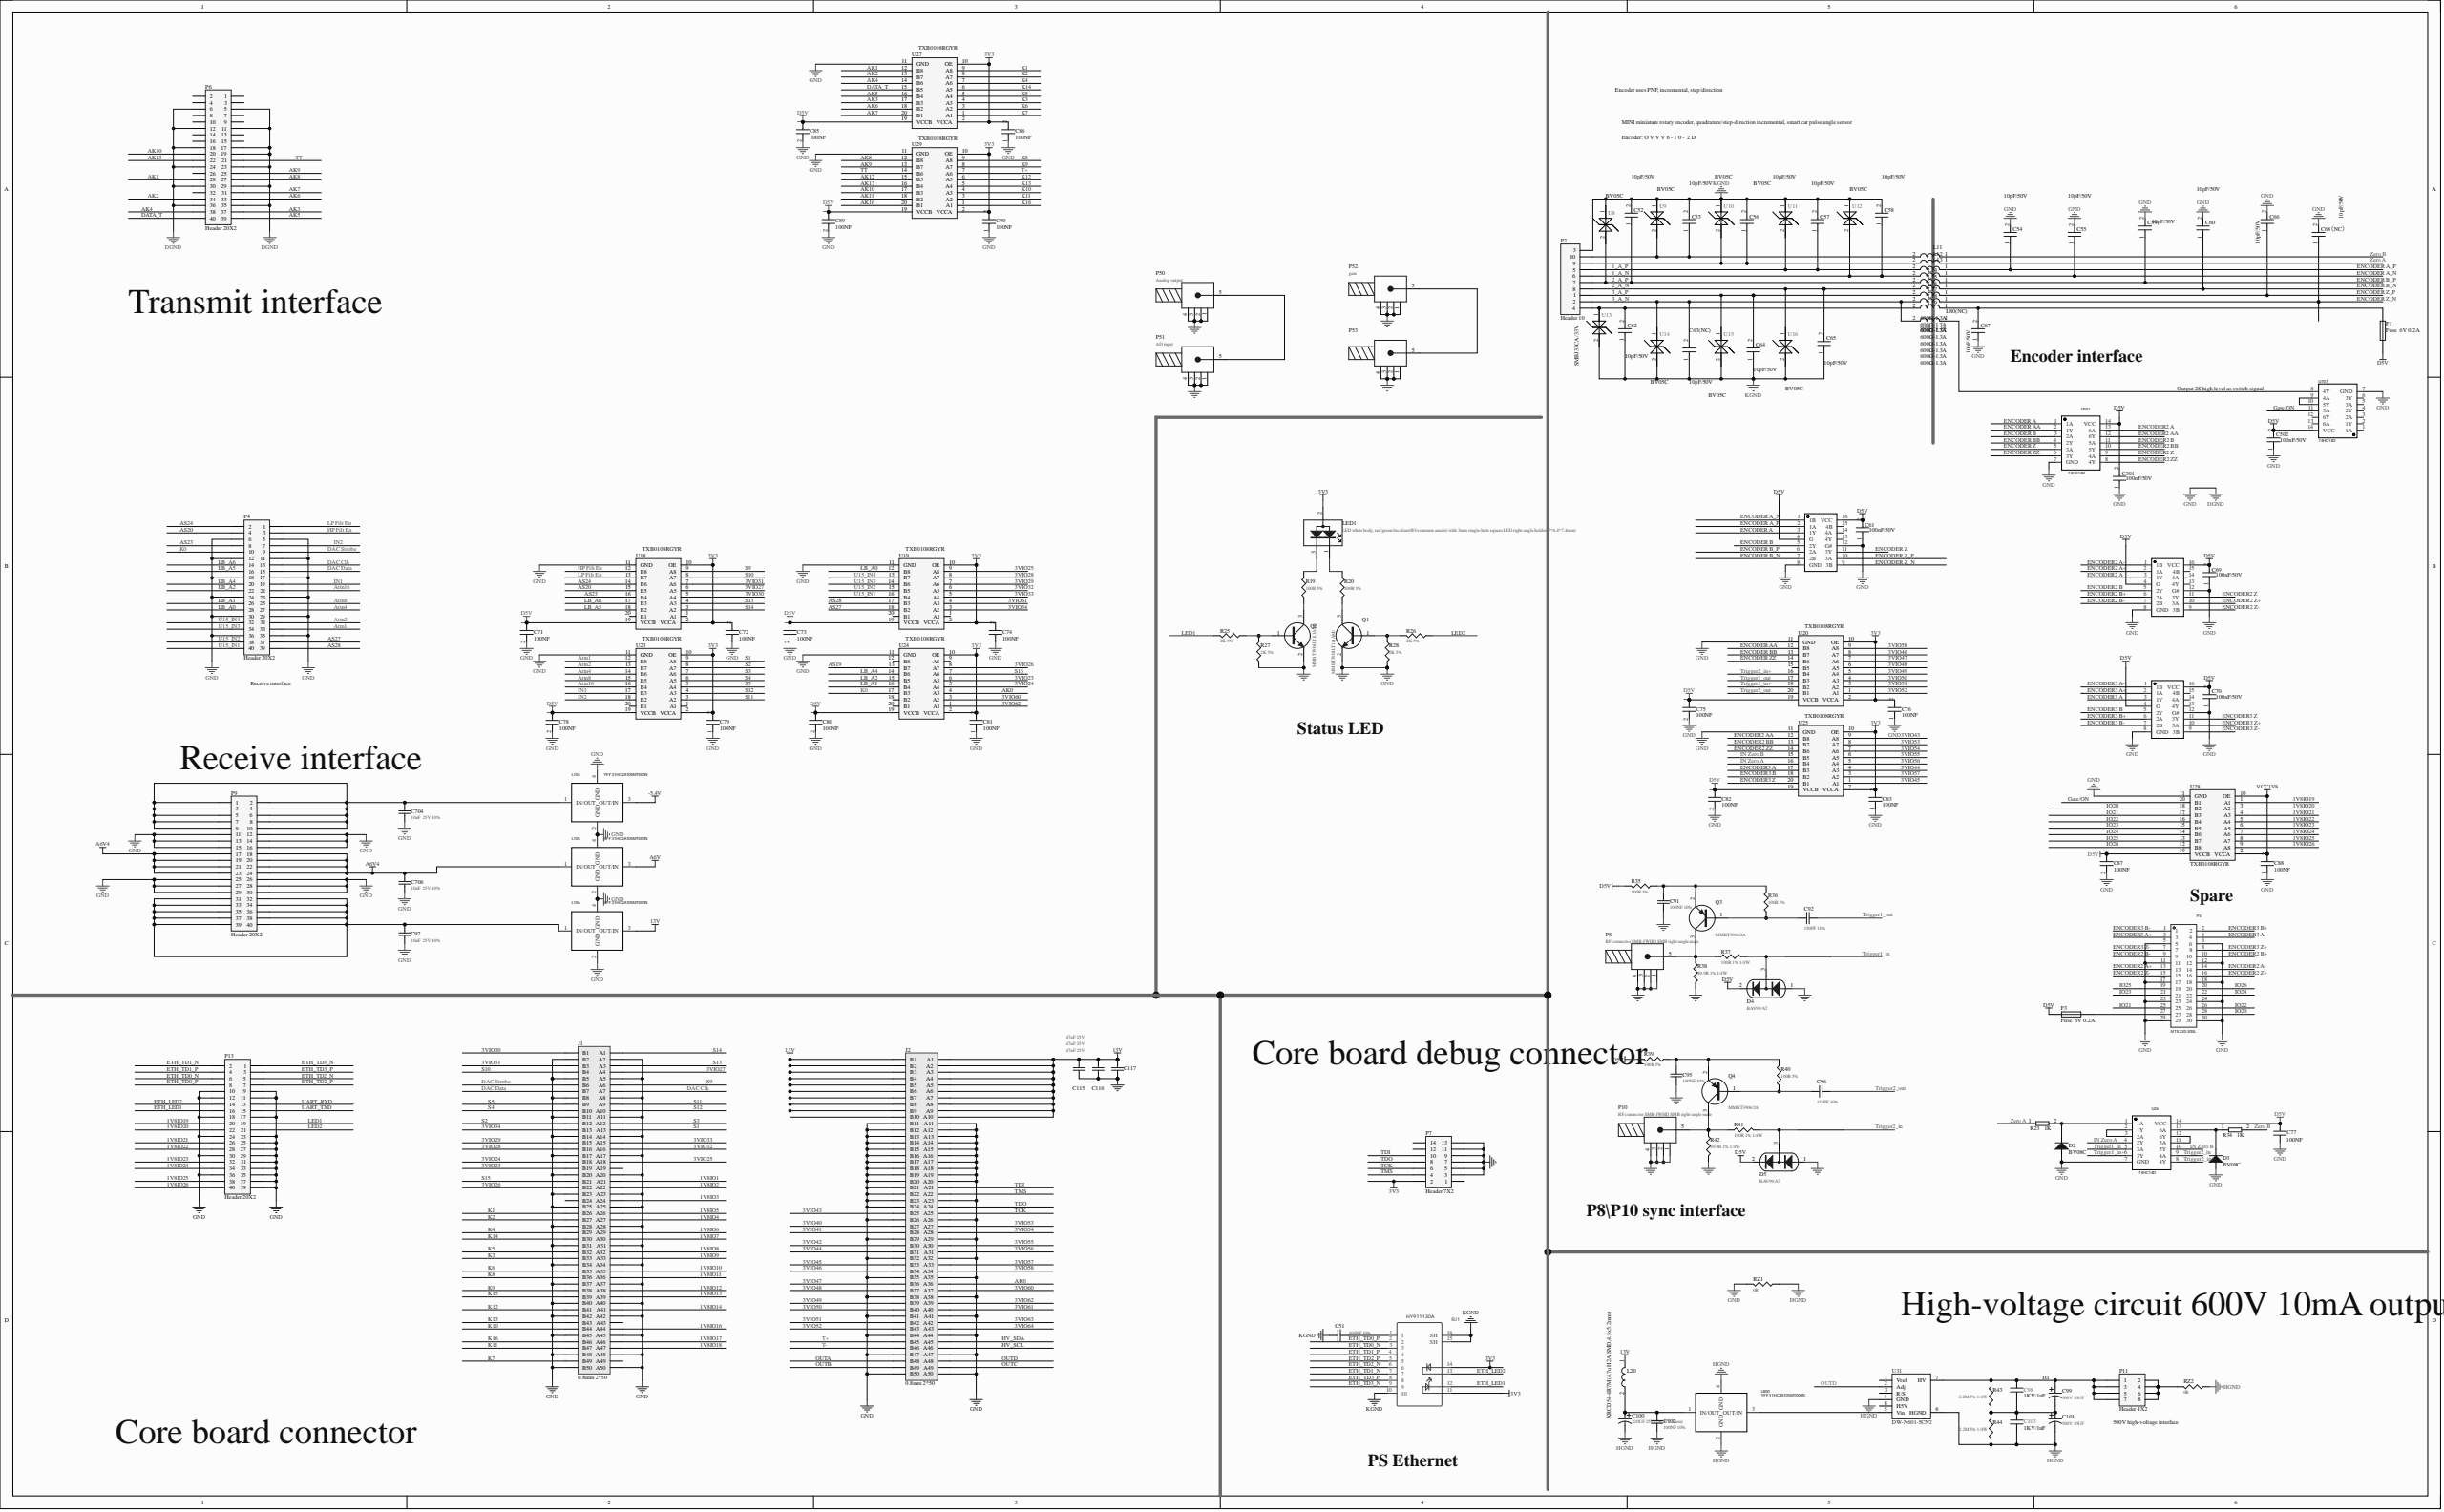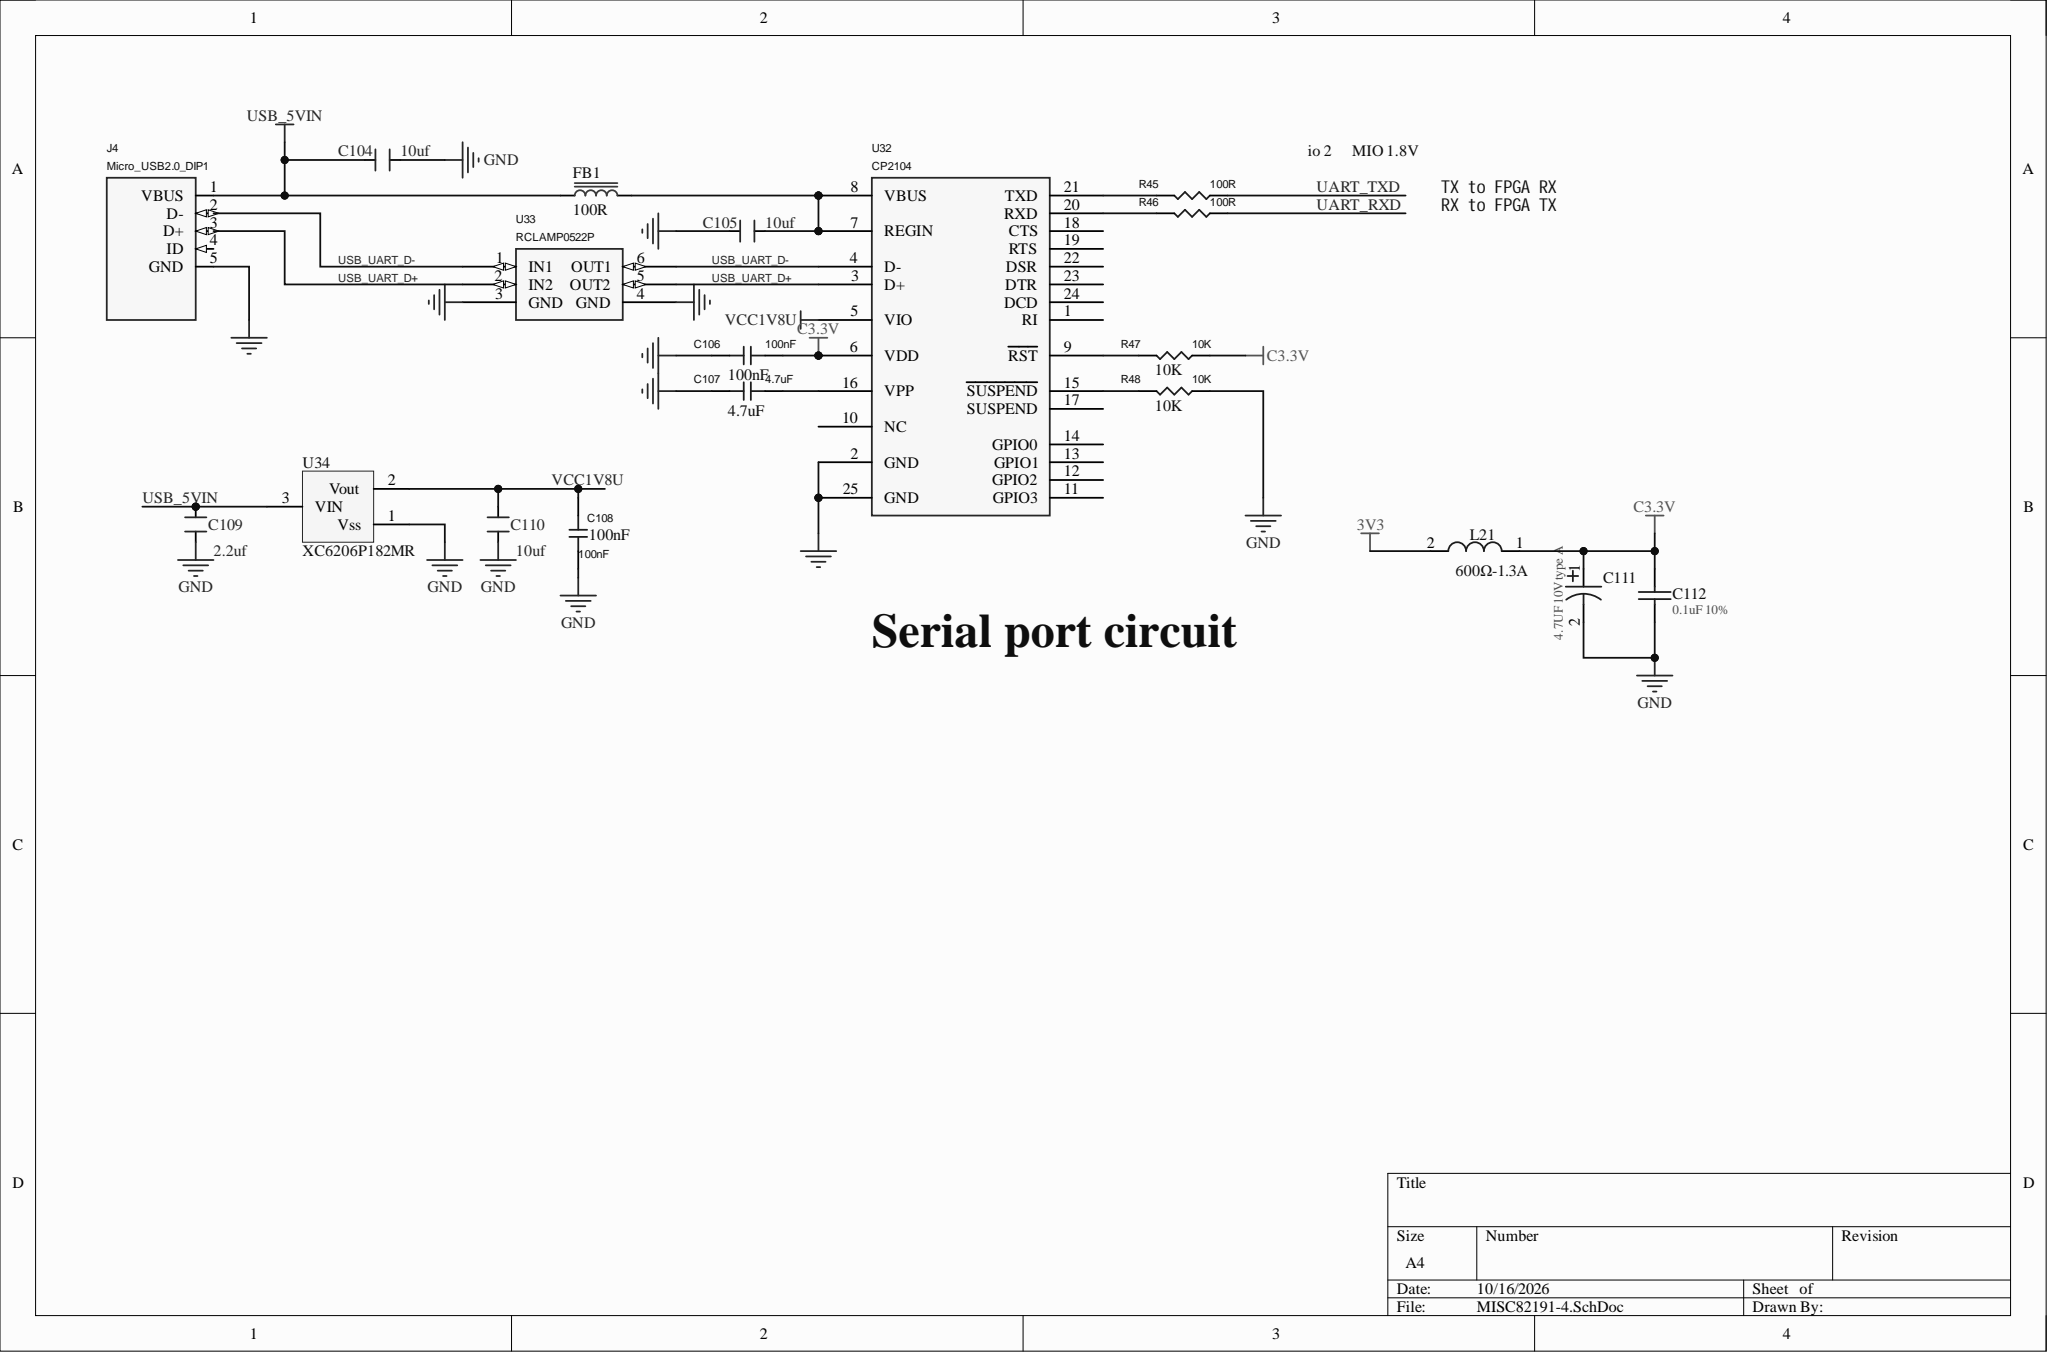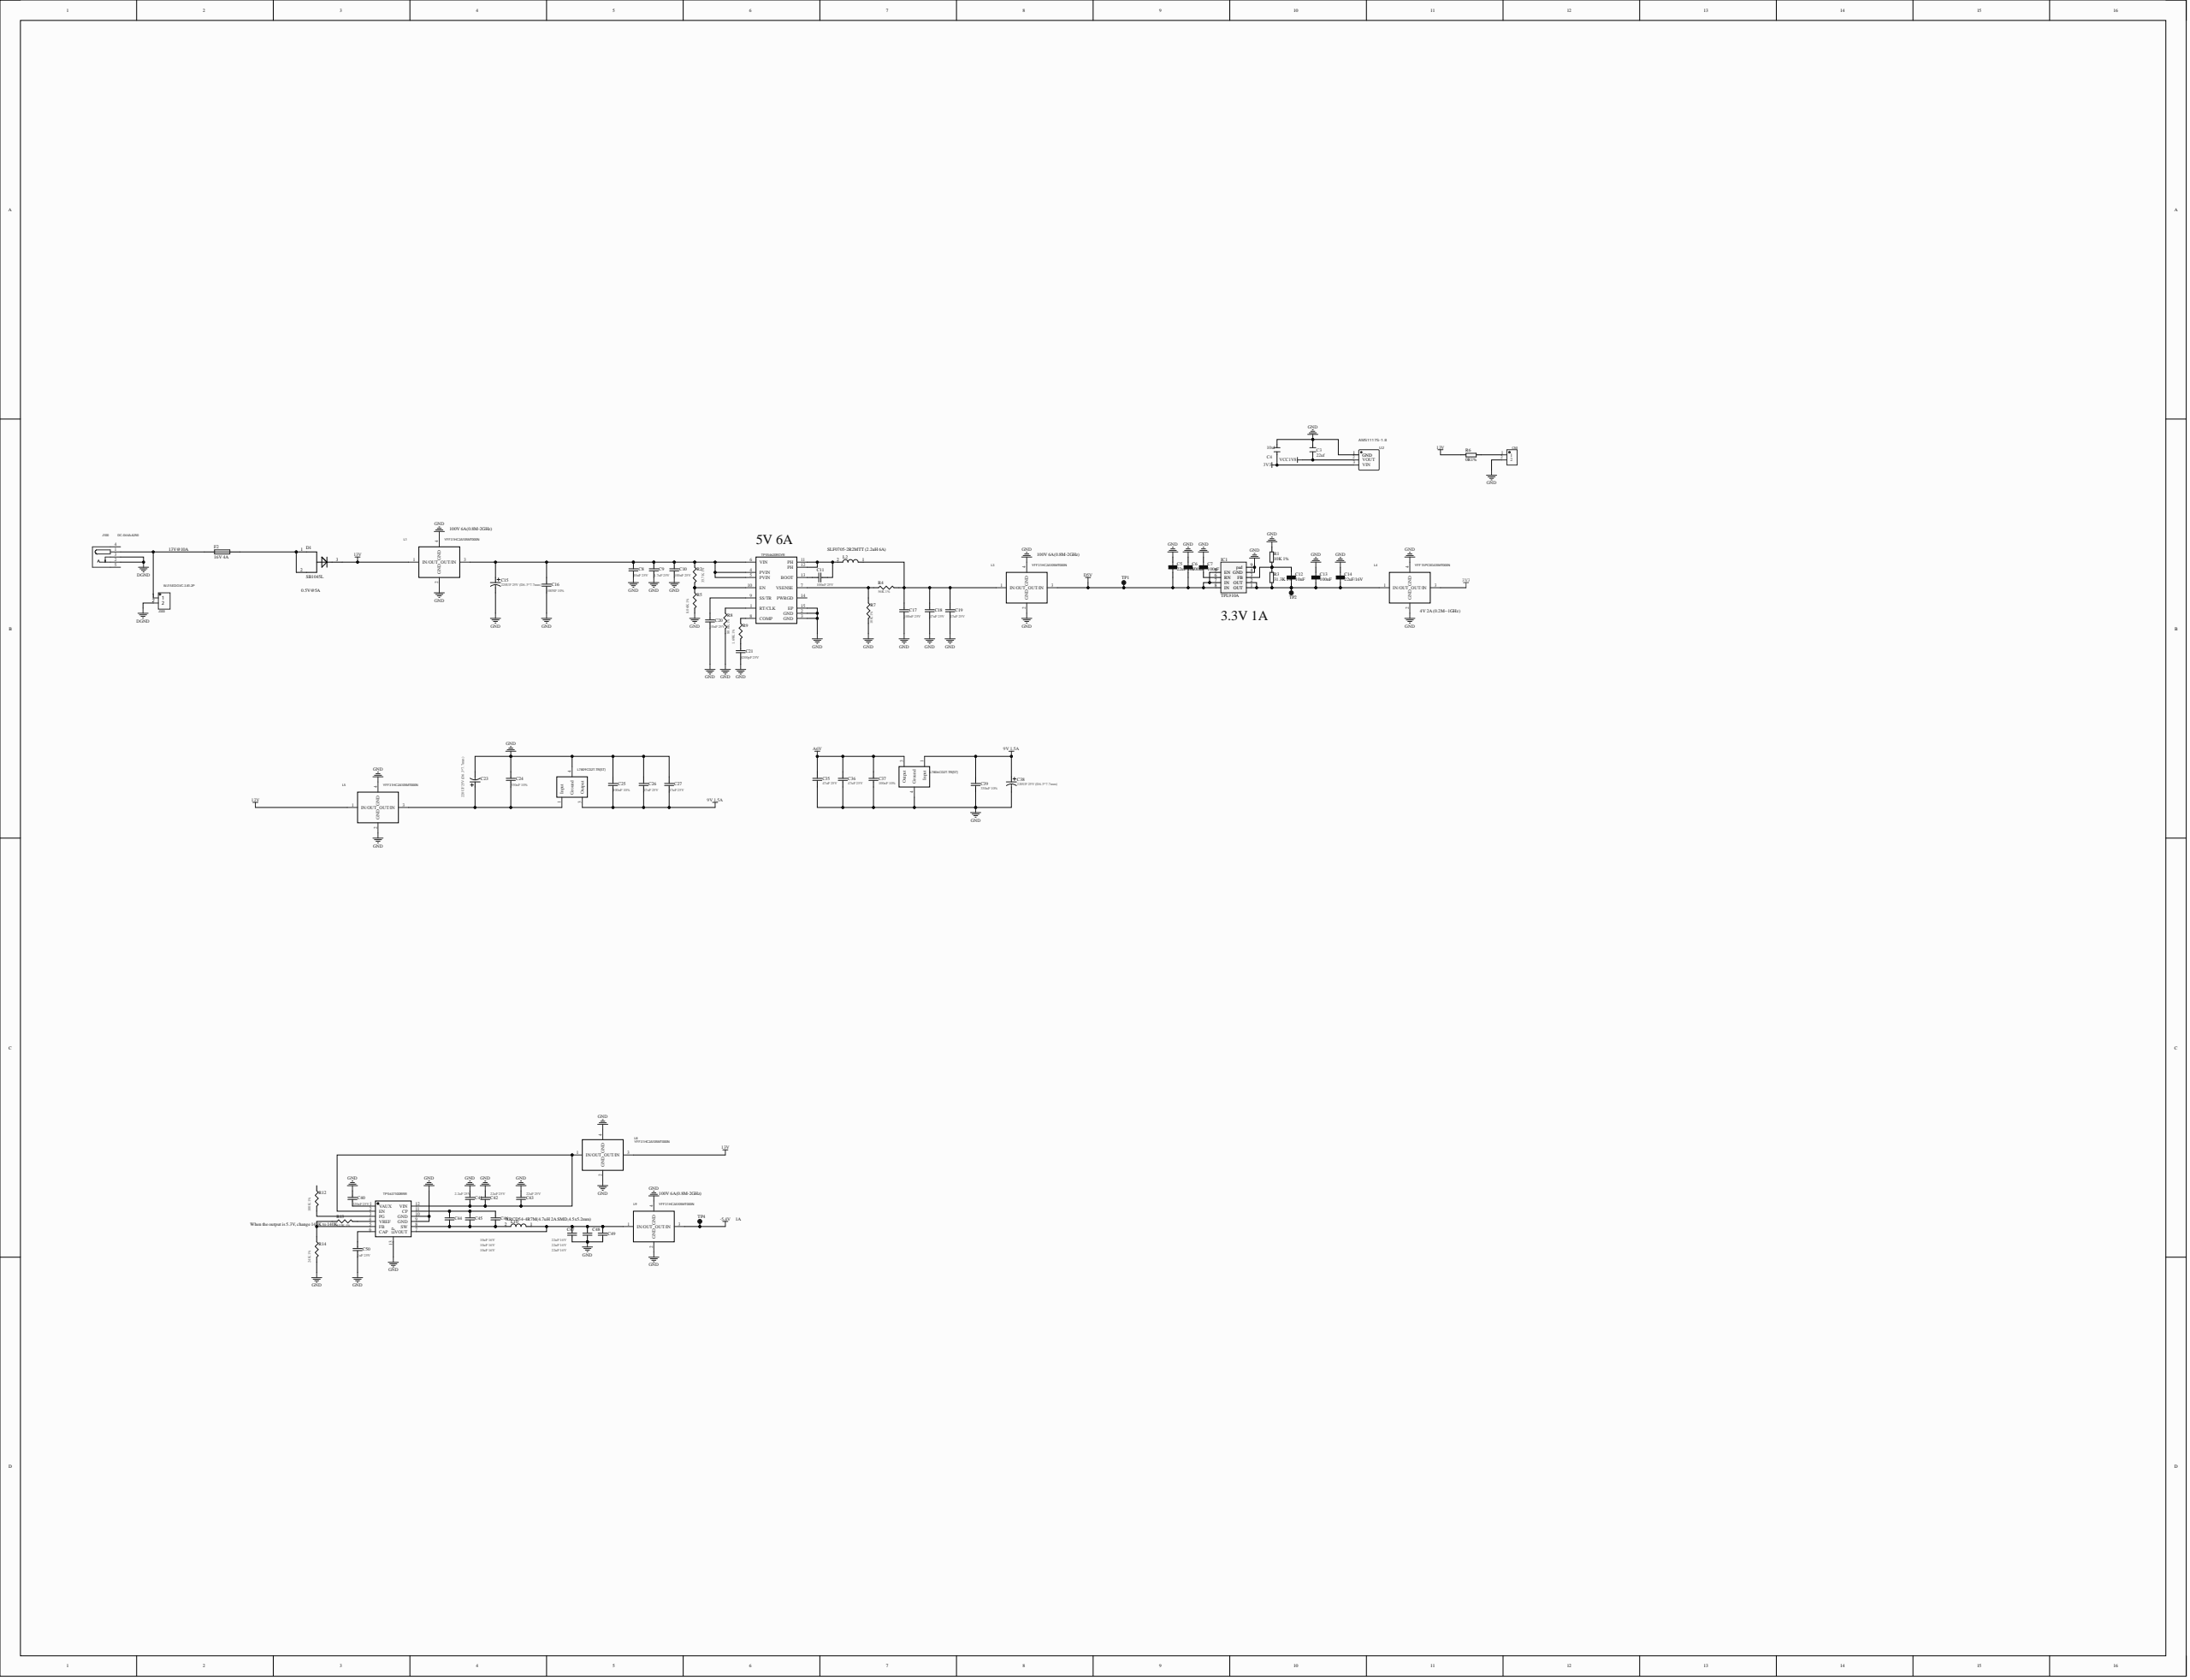Circuit board | Altium Designer | 238 parts | 266 nets
Bill of materials:
Comment,Description,Designator,Footprint,LibRef,Quantity
"22uf","Generic Capacitor","C3","1206","CAPACITOR","1"
"10uf","Generic Capacitor","C4","0805A","CAPACITOR","1"
"22uF/16V","","C5, C14","0805","C1206","2"
"100nF","","C6, C7, C77, C106, C108","0603","C0402, CAP, CAP1","5"
"10uF 25V","Capacitor","C8","0805","CAP","1"
"4.7uF 25V","Capacitor","C9","0603","CAP","1"
"100nF 25V","Capacitor","C10, C11, C17","0603","CAP","3"
"10nF","","C12","0603","C1206","1"
"100nF","","C13","0402","C1206","1"
"220UF 25V (D6.3*7.7mm)","Capacitor","C15, C23, C38, C100","CAP-SMD-6.3","CAPACITOR_1","4"
"100NF 10%","Capacitor","C16","0603","CAP","1"
"47uF 25V","Capacitor","C18, C19, C26, C27, C35, C36, C115, C116, C117","1206","CAP","9"
"10nF 25V","Capacitor","C20","0603","CAP","1"
"8200pF 25V","Capacitor","C21","0603","CAP","1"
"330nF 10%","Capacitor","C24, C39","0805","CAP","2"
"100nF 10%","Capacitor","C25, C37","0805","CAP","2"
"220nF 25V","Capacitor","C40","0603","CAP","1"
"2.2uF 25V","Capacitor","C41","0603","CAP","1"
"22uF 25V","Capacitor","C42, C43","1206","CAP","2"
"10uF 16V","Capacitor","C44, C45, C46","0603","CAP","3"
"22uF 16V","Capacitor","C47, C48, C49","0805","CAP","3"
"1uF 25V","Capacitor","C50","0603","CAP","1"
"100NF 10%","Capacitor","C51","0805A","CAP","1"
"10pF/50V","CC-50V-106-±10%-[1206]","C52, C53, C54, C55, C56, C57, C58, C59, C60, C62, C63(NC), C64, C65, C66, C67, C68（NC）","0603","CAP","16"
"100nF/50V","CC-50V-106-±10%-[1206]","C61, C69, C70, C501, C502","0603","CAP","5"
"100NF","","C71, C72, C73, C74, C75, C76, C78, C79, C80, C81, C82, C83, C85, C86, C87, C88, C89, C90","C0402","CAP","18"
"100NF 10%","Capacitor","C91, C95, C102","0805R","CAP","3"
"150PF 10%","Capacitor","C92, C96","0805R","CAP","2"
"10uF  25V 10%","Capacitor","C97, C704, C706","0805R","CAP","3"
"1KV/1nF","","C98, C103","3225[1210]","CAP","2"
"500V 10UF","Capacitor","C99, C101","CAP-SMD_BD10.0-L10.3-W10.3-LS11.0-R-RD","CAPACITOR","2"
"10uf","Generic Capacitor","C104, C105, C110","0805","CAPACITOR","3"
"4.7uF","","C107","0603","CAP1","1"
"2.2uf","Generic Capacitor","C109","0603","CAPACITOR","1"
"4.7UF 10V type A","Capacitor","C111","1005","CAPACITOR","1"
"0.1uF 10%","Capacitor","C112","0603","CAP","1"
"ZX-XH2.54-2PZZ","","CN1","CONN-TH_2P-P2.50_HX25003-2A","ZX-XH2.54-2PZZ","1"
"SB1045L","","D1","SB1045L","SB1045L","1"
"BV08C","","D2, D3","SOD323","D","2"
"BAV99/A7","Diode","D4, D5","SOT-23","D1","2"
"Fuse  6V 0.2A","Fuse","F1, F3","0805","Fuse 1","2"
"16V 4A","Fuse","F2","1812","Fuse 1","1"
"100R","Generic Ferrite Bead, [NoValue]","FB1, R45, R46","0603","Ferrite Bead, RES1","3"
"TPL910A","3PEAK","IC1","DFN-8_L3.0-W3.0-P0.65-BL-EP2.3","TPL910A","1"
"0.8mm 2*50","","J1, J2","板对板座2*50","0.8mm 2*50","2"
"Micro_USB2.0_DIP1","","J4","MINI-USB-TH_USB-MINI-2","Micro_USB2_0.0_DIP1","1"
"DC-044A-A250","","J100","DC-IN-TH_DC-044A-A250","DC-044A-A250","1"
"WJ15EDGVC-3.81-2P","","J300","CONN-TH_WJ15EDGVC-3.81-2P","WJ15EDGVC-3.81-2P","1"
"YFF31HC2A105MT000N","","L1, L3, L5, L8, L9, L104, L105, L106, L800","FILTER-SMD_4P-L3.2-W1.6-L_YFF31HC","YFF31HC2A105MT000N","9"
"SLF0705-2R2MTT (2.2uH 6A)","","L2","IND-SMD_L7.8-W7.0-A","L","1"
"YFF15PC0G435MT000N","","L4","FILTER-SMD_4P-L1.0-W0.5-L","YFF31HC2A105MT000N","1"
"XRCD54-4R7M(4.7uH 2A SMD,4.5x5.2mm)","","L10, L20","IND-SMD_L7.8-W7.0-A","L","2"
"600Ω-1.3A","BLM18KG601SN-[0603]/Murata","L11, L12, L13, L14, L15, L16, L17, L18, L19, L80(NC)","0805","L","10"
"600Ω-1.3A","BLM18KG601SN-[0603]/Murata","L21","0603","L","1"
"LED white body, red/green bicolour(F3/common anode) with 3mm single-hole square LED right-angle holder(7*6.4*7.4mm)","","LED1","DIP3B","LED_2","1"
"Header 10","Header, 10-Pin","P2","2B-10","Header 10","1"
"MTE220-30SL","","P3","CONN-TH_MTE220-30SL","MTE220-30SL","1"
"Header 20X2","Header, 20-Pin, Dual row","P4, P6, P9, P13","N0.8mm/40Pin-Plug","Header 20X2","4"
"Header 7X2","Header, 7-Pin, Dual row","P7","IDC-TH_14P-P2.54-V-R2-C7-S2.54","Header 7X2","1"
"RF connector SMB-JWHD SMB right-angle male","","P8, P10","DIP-P","JA1","2"
"Header 4X2","Header, 4-Pin, Dual row","P11","N0.8mm/8Pin-SOCKET","Header 4X2","1"
"Analog output","","P50","DIP-P","JA1","1"
"AD input","","P51","DIP-P","JA1","1"
"gain","","P52","DIP-P","JA1","1"
"","","P53","DIP-P","JA1","1"
"MMBT3904LT1(1AM)","NPN Transistor","Q1, Q2","SOT23","NPN","2"
"MMBT3906/2A","PNP Transistor","Q3, Q4","SOT-23","PNP","2"
"10K 1%","","R1, R7","0603","R0603, RES1","2"
"35.7K 1%","","R2","0603","RES1","1"
"31.3K 1%","","R3","0603","R0603","1"
"56K 1%","","R4","0603","RES1","1"
"8.06K 1%","","R5","0603","RES1","1"
"0R1%","","R6","0805","R0603","1"
"80.6K 1%","","R8","0603","RES1","1"
"1.69K 1%","","R9","0603","RES1","1"
"100K 1%","","R12","0603","RES1","1"
"143K 1%","","R13","0603","RES1","1"
"24K 1%","","R14","0603","RES1","1"
"100R 5%","","R19, R20","0603A","RES1","2"
"1K","","R23, R34","0402","RES","2"
"2K 5%","","R25, R26, R27, R28","0603A","RES1","4"
"100R 5%","","R35, R36, R39, R40","0805R","RES1","4"
"100R 1% 1/4W","","R37, R41","AXIAL-0.45","RES1","2"
"49.9R 1% 1/4W","","R38, R42","AXIAL-0.5","RES1","2"
"2.2M 5% 1/4W","","R43, R44","AXIAL-0.5","RES1","2"
"10K","","R47, R48","0603","RES1","2"
"HY911130A","","RJ1","HY911130A","HY911130A","1"
"0R","","RZ1, RZ2","0805R","RES1","2"
"","","TP1, TP2, TP4","TP1","TEST_2","3"
"AMS1117S-1.8","","U2","SOT-89-3_L4.5-W2.5-P1.50-LS4.2-BR","AMS1117S-3.3","1"
"TPS54620RGYR","","U3","VQFN-14_L3.5-W3.5-P0.50-BL-EP_TPS54622RHLT","TPS54620RGYR","1"
"L7809CD2T-TR(ST)","","U5","TO-263-2_L10.0-W9.1-P5.08-LS15.2-TL","L7809CD2T-TR","1"
"L7806CD2T-TR(ST)","","U6","TO-263-2_L10.0-W9.1-P5.08-LS15.2-TL","L7809CD2T-TR","1"
"TPS63710DRRR","","U7","TDFN-12_L3.0-W3.0-P0.50-BL-EP","TPS63710DRRR","1"
"BV05C","BV05C-[SOD-323]/Bencent","U8, U9, U10, U11, U12, U14, U15, U16","SOD-323","SMAJ18CA 18V","8"
"SMBJ33CA /33V","","U13","DO-214AC(SMA)","SMAJ18CA 18V","1"
"AM26LV32EIPWR","","U17, U21, U22","TSSOP-16_L5.0-W4.4-P0.65-LS6.4-BL","AM26LV32EIPWR","3"
"TXB0108RGYR","","U18, U19, U20, U23, U24, U25, U27, U28, U29","QFN20","TXB0108RGYR","9"
"74HC14D","","U26, U501, U707","SO-14","74HC14D,653","3"
"DW-N601-5CN2","","U31","DW-N601-5CN2","DW-N601-5CN2","1"
"CP2104","","U32","QFN-24_L4.0-W4.0-P0.50-BL-EP2.7","CP2104","1"
"RCLAMP0522P","","U33","DFN-1610-6_L1.6-W1.0-P0.50-BL","RCLAMP0522P","1"
"XC6206P182MR","","U34","SOT-23-3_L2.9-W1.6-P1.90-LS2.8-BR","XC6206P332MR","1"
Netlist (net: part-pin ...):
Zero B: L11-1 R34-2
Zero A: L12-1 R23-1
VCC1V8U: C108-2 C110-2 U32-5 U34-2
VCC1V8: C3-1 C88-2 U2-2 U28-2 U28-10
USB_UART_D-: J4-2 U32-4 U33-1 U33-6
USB_UART_D+: J4-3 U32-3 U33-2 U33-5
USB_5VIN: C104-2 C109-2 FB1-1 J4-1 U34-3
UART_TXD: P13-15 R45-2
UART_RXD: P13-13 R46-2
U15_IN4: P4-32 U19-13
U15_IN3: P4-34 U19-14
U15_IN2: P4-38 U19-15
U15_IN1: P4-40 U19-16
TT: P6-21 U29-14
Trigger2_out: C96-1 U20-20
Trigger2_in+: U20-16 U26-8
Trigger2_in: D5-3 R41-1 U26-9
Trigger1_out: C92-1 U20-17
Trigger1_in+: U20-18 U26-6
Trigger1_in: D4-3 R37-1 U26-5
TMS: J2-A22 P7-4
TDO: J2-A24 P7-8
TDI: J2-A21 P7-10
TCK: J2-A25 P7-6
T+: J2-B45 U29-7
S15: J1-B21 U24-7
S14: J1-A1 U18-3
S13: J1-A3 U18-4
S12: J1-A10 U23-4
S11: J1-A9 U23-3
S10: J1-B4 U18-8
S9: J1-A6 U18-9
S5: J1-B9 U23-5
S4: J1-B10 U23-6
S3: J1-A12 U23-7
S2: J1-B12 U23-8
S1: J1-A13 U23-9
OUTD: J2-A48 U31-2
NetU707_9: U707-9 U707-10
NetU26_11: U26-11 U26-12
NetU26_2: U26-2 U26-3
NetR48_1: R48-1 U32-15
NetR47_1: R47-1 U32-9
NetR46_1: R46-1 U32-20
NetR45_1: R45-1 U32-21
NetR13_2: R13-2 U7-4
NetR13_1: R13-1 R14-1 U7-5
NetR12_2: R12-2 U7-3
NetR9_1: R9-1 U3-8
NetR8_1: R8-1 U3-1
NetR4_1: R4-1 R7-1 U3-7
NetR2_2: R2-2 R5-1 U3-10
NetQ2_3: Q2-3 R19-1
NetQ2_1: Q2-1 R25-2 R27-2
NetQ1_3: Q1-3 R20-1
NetQ1_1: Q1-1 R26-2 R28-2
NetP52_5: P52-5 P53-5
NetP50_5: P50-5 P51-5
NetP11_2: P11-2 P11-4 P11-6 P11-8 RZ2-2
NetP10_5: P10-5 Q4-3 R41-2 R42-2
NetP8_5: P8-5 Q3-3 R37-2 R38-2
NetLED1_3: LED1-3 R19-2
NetLED1_1: LED1-1 R20-2
NetL800_3: L800-3 U31-5
NetL80(NC)_1: L80(NC)-1 U707-8
NetF3_1: F3-1 P3-27
NetF2_1: F2-1 J100-1 J300-1
NetD3_2: D3-2 R34-1 U26-13
NetD2_2: D2-2 R23-2 U26-1
NetD1_1: D1-1 D1-2 F2-2
NetCN1_1: CN1-1 R6-2
NetC704_2: C704-2 L104-1 P9-1 P9-2 P9-3 P9-4 P9-5 P9-6 P9-7 P9-8 P9-9 P9-10
NetC107_2: C107-2 U32-16
NetC105_1: C105-1 FB1-2 U32-7 U32-8
NetC100_1: C100-1 C102-1 L20-2 L800-1
NetC98_2: C98-2 C99-2 C101-1 C103-1 R43-1 R44-2
NetC97_1: C97-1 L106-1 P9-31 P9-32 P9-33 P9-34 P9-35 P9-36 P9-37 P9-38 P9-39 P9-40
NetC96_2: C96-2 Q4-1 R40-2
NetC95_1: C95-1 Q4-2 R39-1 R40-1
NetC92_2: C92-2 Q3-1 R36-2
NetC91_1: C91-1 Q3-2 R35-1 R36-1
NetC67_2: C67-2 F1-1 L19-1
NetC62_2: C62-2 L19-2 P2-4 U13-1
NetC56_1: C56-1 L12-2 P2-9 U10-2
NetC53_1: C53-1 L11-2 P2-10 U9-2
NetC51_1: C51-1 RJ1-1
NetC50_1: C50-1 U7-6
NetC47_2: C47-2 C48-2 C49-2 L9-1 L10-1 U7-7
NetC44_2: C44-2 C45-2 C46-2 U7-11
NetC44_1: C44-1 C45-1 C46-1 L10-2 U7-8
NetC41_1: C41-1 C42-1 C43-1 L8-1 U7-2 U7-12
NetC40_2: C40-2 U7-1
NetC23_1: C23-1 C24-2 L5-3 U5-1
NetC21_1: C21-1 R9-2
NetC20_1: C20-1 U3-9
NetC17_1: C17-1 C18-1 C19-1 L2-1 L3-1 R4-2
NetC12_2: C12-2 C13-2 C14-2 IC1-1 IC1-2 L4-1 R3-2 TP2-1
NetC12_1: C12-1 IC1-3 R1-2 R3-1
NetC11_2: C11-2 L2-2 U3-11 U3-12
NetC11_1: C11-1 U3-13
NetC8_1: C8-1 C9-1 C10-1 C15-1 C16-1 L1-3 R2-1 U3-4 U3-5 U3-6
NetC7_2: C7-2 IC1-6
LP Filt En: P4-1 U18-13
LED2: P13-21 R26-1
LED1: P13-19 R25-1
LB_A6: P4-14 U18-17
LB_A5: P4-16 U18-18
LB_A4: P4-20 U24-14
LB_A2: P4-22 U24-15
LB_A1: P4-26 U24-16
LB_A0: P4-28 U19-12
KGND: C51-2 C52-2 C53-2 C56-2 C57-2 C58-2 C62-1 C63(NC)-1 C64-1 C65-1 P2-3 RJ1-10 RJ1-15 RJ1-16 U8-1 U9-1 U10-1 U11-1 U12-1 U13-2 U14-2 U15-2 U16-2
K16: J1-B46 U29-1
K14: J1-B30 U27-6
K13: J1-B43 U29-5
K12: J1-B41 U29-6
K11: J1-B47 U29-3
K10: J1-B44 U29-4
K9: J1-B38 U29-8
K8: J1-B36 U29-9
K7: J1-B49 U27-1
K6: J1-B35 U27-3
K5: J1-B32 U27-5
K4: J1-B29 U27-7
K3: J1-B33 U27-4
K2: J1-B27 U27-8
K1: J1-B26 U27-9
K0: P4-10 U24-17
IO26: P3-20 U28-12
IO25: P3-19 U28-13
IO24: P3-22 U28-14
IO23: P3-21 U28-15
IO22: P3-26 U28-16
IO21: P3-25 U28-17
IO20: P3-28 U28-18
IN Zero B: U25-15 U26-10
IN Zero A: U25-16 U26-4
IN2: P4-7 U23-18
IN1: P4-19 U23-17
HT: C98-1 C99-1 P11-1 P11-3 P11-5 P11-7 R43-2 U31-7
HP Filt En: P4-3 U18-12
HGND: C100-2 C101-2 C102-2 C103-2 L800-2 L800-4 R44-1 RZ1-1 RZ2-1 U31-4 U31-6
Gate/ON: U28-20 U707-11
ETH_TD3_P: P13-3 RJ1-8
ETH_TD3_N: P13-1 RJ1-9
ETH_TD2_P: P13-7 RJ1-5
ETH_TD2_N: P13-5 RJ1-6
ETH_TD1_P: P13-4 RJ1-4
ETH_TD1_N: P13-2 RJ1-7
ETH_TD0_P: P13-8 RJ1-2
ETH_TD0_N: P13-6 RJ1-3
ETH_LED2: P13-14 RJ1-13
ETH_LED1: P13-16 RJ1-12
ENCODER ZZ: U20-14 U501-6
ENCODER Z_P: C66-1 L17-1 U17-10
ENCODER Z_N: C68（NC）-1 L18-1 U17-9
ENCODER Z: U17-11 U501-5
ENCODER BB: U20-13 U501-4
ENCODER B_P: C59-1 L15-1 U17-6
ENCODER B_N: C60-1 L16-1 U17-7
ENCODER B: U17-5 U501-3
ENCODER AA: U20-12 U501-2
ENCODER A_P: C54-1 L13-1 U17-2
ENCODER A_N: C55-1 L14-1 U17-1
ENCODER A: U17-3 U501-1
ENCODER3 Z-: P3-7 U22-9
ENCODER3 Z+: P3-8 U22-10
ENCODER3 Z: U22-11 U25-20
ENCODER3 B-: P3-1 U22-7
ENCODER3 B+: P3-2 U22-6
ENCODER3 B: U22-5 U25-18
ENCODER3 A-: P3-4 U22-1
ENCODER3 A+: P3-3 U22-2
ENCODER3 A: U22-3 U25-17
ENCODER2 ZZ: U25-14 U501-8
ENCODER2 Z-: P3-15 U21-9
ENCODER2 Z+: P3-16 U21-10
ENCODER2 Z: U21-11 U501-9
ENCODER2 BB: U25-13 U501-10
ENCODER2 B-: P3-9 U21-7
ENCODER2 B+: P3-10 U21-6
ENCODER2 B: U21-5 U501-11
ENCODER2 AA: U25-12 U501-12
ENCODER2 A-: P3-14 U21-1
ENCODER2 A+: P3-13 U21-2
ENCODER2 A: U21-3 U501-13
DGND: C3-2 C4-1 C5-1 C6-1 C7-1 C8-2 C9-2 C10-2 C13-1 C14-1 C15-2 C16-2 C17-2 C18-2 C19-2 C20-2 C21-2 C23-2 C24-1 C25-1 C26-1 C27-1 C35-1 C36-1 C37-1 C38-2 C39-1 C40-1 C41-2 C42-2 C43-2 C47-1 C48-1 C49-1 C50-2 C54-2 C55-2 C59-2 C60-2 C61-1 C66-2 C67-1 C68（NC）-2 C69-1 C70-1 C71-2 C72-1 C73-2 C74-1 C75-2 C76-1 C77-1 C78-2 C79-1 C80-2 C81-1 C82-2 C83-1 C85-2 C86-1 C87-2 C88-1 C89-2 C90-1 C91-2 C95-2 C97-2 C104-1 C105-2 C106-1 C107-1 C108-1 C109-1 C110-1 C111-2 C112-2 C115-2 C116-1 C117-1 C501-1 C502-1 C704-1 C706-1 CN1-2 D2-1 D3-1 D4-1 D5-1 IC1-4 IC1-9 J1-A2 J1-A5 J1-A8 J1-A11 J1-A14 J1-A17 J1-A20 J1-A23 J1-A25 J1-A28 J1-A31 J1-A34 J1-A37 J1-A40 J1-A42 J1-A45 J1-A48 J1-A50 J1-B2 J1-B5 J1-B8 J1-B11 J1-B14 J1-B17 J1-B20 J1-B23 J1-B25 J1-B28 J1-B31 J1-B34 J1-B37 J1-B40 J1-B42 J1-B45 J1-B48 J1-B50 J2-A11 J2-A12 J2-A13 J2-A14 J2-A15 J2-A16 J2-A17 J2-A18 J2-A19 J2-A20 J2-A23 J2-A26 J2-A29 J2-A32 J2-A35 J2-A38 J2-A41 J2-A44 J2-A47 J2-A50 J2-B11 J2-B12 J2-B13 J2-B14 J2-B15 J2-B16 J2-B17 J2-B18 J2-B19 J2-B20 J2-B21 J2-B22 J2-B23 J2-B24 J2-B26 J2-B29 J2-B32 J2-B35 J2-B38 J2-B41 J2-B44 J2-B47 J2-B50 J4-5 J100-2 J100-3 J300-2 L1-2 L1-4 L3-2 L3-4 L4-2 L4-4 L5-2 L5-4 L8-2 L8-4 L9-2 L9-4 L104-2 L104-4 L105-2 L105-4 L106-2 L106-4 P3-5 P3-6 P3-11 P3-12 P3-17 P3-18 P3-23 P3-24 P3-29 P3-30 P4-5 P4-6 P4-11 P4-12 P4-17 P4-18 P4-23 P4-24 P4-29 P4-30 P4-35 P4-36 P6-5 P6-6 P6-11 P6-12 P6-17 P6-18 P6-19 P6-23 P6-24 P6-29 P6-30 P6-35 P6-36 P7-3 P7-5 P7-7 P7-9 P7-11 P7-13 P8-1 P8-2 P8-3 P8-4 P9-11 P9-12 P9-13 P9-14 P9-15 P9-16 P9-25 P9-26 P9-27 P9-28 P9-29 P9-30 P10-1 P10-2 P10-3 P10-4 P13-9 P13-10 P13-11 P13-12 P13-17 P13-18 P13-23 P13-24 P13-25 P13-27 P13-29 P13-30 P13-31 P13-33 P13-35 P13-36 P13-37 P13-39 P50-1 P50-2 P50-3 P50-4 P51-1 P51-2 P51-3 P51-4 P52-1 P52-2 P52-3 P52-4 P53-1 P53-2 P53-3 P53-4 Q1-2 Q2-2 R1-1 R5-2 R7-2 R8-2 R14-2 R27-1 R28-1 R38-1 R42-1 R48-2 RZ1-2 U2-1 U3-2 U3-3 U3-15 U5-4 U6-4 U7-9 U7-10 U7-13 U17-8 U17-12 U18-11 U19-11 U20-11 U21-8 U21-12 U22-8 U22-12 U23-11 U24-11 U25-11 U26-7 U27-11 U28-11 U29-11 U32-2 U32-25 U33-3 U33-4 U34-1 U501-7 U707-7
DATA_T: P6-40 U27-15
DAC Strobe: J1-B6 P4-9
DAC Data: J1-B7 P4-15
DAC Clk: J1-A7 P4-13
D5V: C5-2 C6-2 C61-2 C69-2 C70-2 C71-1 C73-1 C75-1 C77-2 C78-1 C80-1 C82-1 C85-1 C87-1 C89-1 C501-2 C502-2 D4-2 D5-2 F1-2 F3-2 IC1-5 IC1-7 IC1-8 L3-3 R35-2 R39-2 TP1-1 U17-4 U17-16 U18-19 U19-19 U20-19 U21-4 U21-16 U22-4 U22-16 U23-19 U24-19 U25-19 U26-14 U27-19 U28-19 U29-19 U501-14 U707-14
C3.3V: C106-2 C111-1 C112-1 L21-1 R47-2 U32-6
Attn16: P4-21 U23-16
Attn8: P4-25 U23-15
Attn4: P4-27 U23-14
Attn2: P4-31 U23-13
Attn1: P4-33 U23-12
AS28: P4-39 U19-17
AS27: P4-37 U19-18
AS24: P4-2 U18-14
AS23: P4-8 U18-16
AS20: P4-4 U18-15
AK13: P6-22 U29-16
AK10: P6-20 U29-17
AK9: P6-25 U29-13
AK8: P6-27 U29-12
AK7: P6-31 U27-20
AK6: P6-33 U27-18
AK5: P6-39 U27-16
AK4: P6-38 U27-14
AK3: P6-37 U27-17
AK2: P6-34 U27-13
AK1: P6-28 U27-12
AK0: J2-A36 U24-4
A6V4: C706-2 L105-1 P9-17 P9-18 P9-19 P9-20 P9-21 P9-22 P9-23 P9-24
A6V: C35-2 C36-2 C37-2 L105-3 U6-3
-5.4V: L9-3 L104-3 TP4-1
13V: C115-1 C116-2 C117-2 D1-3 J2-A1 J2-A2 J2-A3 J2-A4 J2-A5 J2-A6 J2-A7 J2-A8 J2-A9 J2-A10 J2-B1 J2-B2 J2-B3 J2-B4 J2-B5 J2-B6 J2-B7 J2-B8 J2-B9 J2-B10 L1-1 L5-1 L8-3 L20-1 L106-3 R6-1
9V 1.5A: C25-2 C26-2 C27-2 C38-1 C39-2 U5-3 U6-1
3VIO62: J2-A39 U24-1
3VIO61: J2-A40 U19-4
3VIO60: J2-A37 U24-3
3VIO58: J2-A34 U20-9
3VIO57: J2-A33 U25-3
3VIO56: J2-A31 U25-5
3VIO55: J2-A30 U25-6
3VIO54: J2-A28 U25-7
3VIO53: J2-A27 U25-8
3VIO52: J2-B43 U20-1
3VIO51: J2-B42 U20-3
3VIO50: J2-B40 U20-4
3VIO49: J2-B39 U20-5
3VIO48: J2-B37 U20-6
3VIO47: J2-B36 U20-7
3VIO46: J2-B34 U20-8
3VIO45: J2-B33 U25-1
3VIO44: J2-B31 U25-4
3VIO43: J2-B25 U25-9
3VIO34: J1-B13 U19-3
3VIO33: J1-A15 U19-5
3VIO32: J1-A16 U19-6
3VIO31: J1-B3 U18-7
3VIO30: J1-B1 U18-5
3VIO29: J1-B15 U19-7
3VIO28: J1-B16 U19-8
3VIO27: J1-A4 U18-6
3VIO26: J1-B22 U24-8
3VIO25: J1-A18 U19-9
3VIO24: J1-B18 U24-5
3VIO23: J1-B19 U24-6
3V3: C4-2 C72-2 C74-2 C76-2 C79-2 C81-2 C83-2 C86-2 C90-2 L4-3 L21-2 LED1-2 P7-2 RJ1-11 RJ1-14 U2-3 U18-2 U18-10 U19-2 U19-10 U20-2 U20-10 U23-2 U23-10 U24-2 U24-10 U25-2 U25-10 U27-2 U27-10 U29-2 U29-10
3_A_P: C64-2 L17-2 P2-1 U15-1
3_A_N: C63(NC)-2 L18-2 L80(NC)-2 P2-2 U14-1
2_A_P: C52-1 L15-2 P2-7 U8-2
2_A_N: C65-2 L16-2 P2-8 U16-1
1V8IO26: P13-40 U28-9
1V8IO25: P13-38 U28-8
1V8IO24: P13-34 U28-7
1V8IO23: P13-32 U28-6
1V8IO22: P13-28 U28-5
1V8IO21: P13-26 U28-4
1V8IO20: P13-22 U28-3
1V8IO19: P13-20 U28-1
1_A_P: C57-1 L13-2 P2-5 U11-2
1_A_N: C58-1 L14-2 P2-6 U12-2